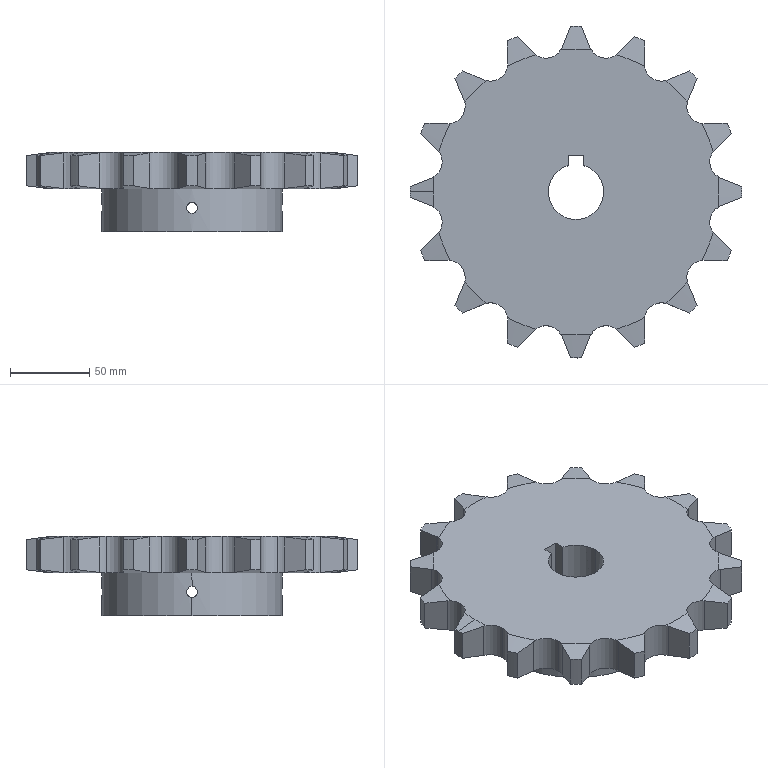Part | STEP file | 24A16T | 1 solid | 124 faces | box 210 x 210 x 50 mm | volume 858195 mm3 | cylinder 52 | plane 38 | cone 34 | commonest cylinder face diameters 22 x22 210 x17 6.8 x8 35 x3 114 x2